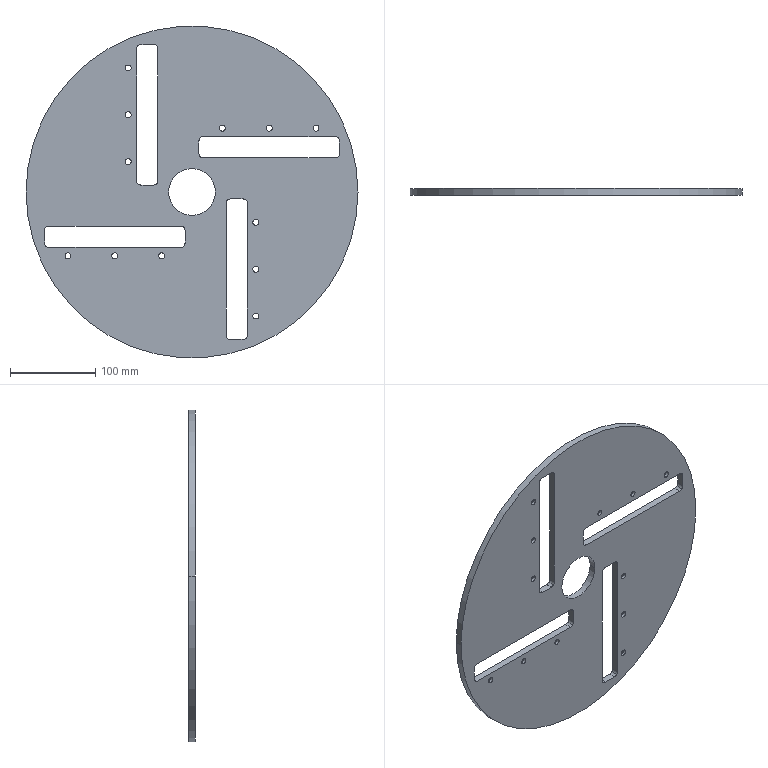Part | SolidWorks | 1 solid | 102 faces | box 390 x 8 x 390 mm | volume 797841 mm3 | cylinder 60 | cone 24 | plane 18 | commonest cylinder face diameters 10 x32 7 x24 55 x2 390 x2